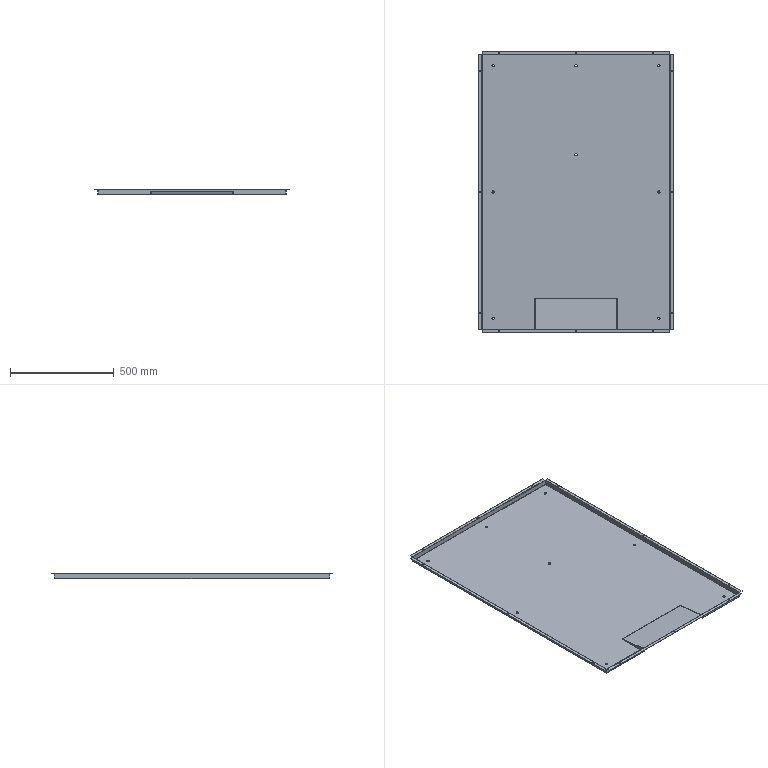Part | SolidWorks | 2 solids | 170 faces | box 940 x 1360 x 25.087 mm | volume 1376149 mm3 | plane 90 | cylinder 68 | spline 12 | commonest cylinder face diameters 7 x30 11 x16 0.4 x9 2.4 x9 2 x2 4 x2